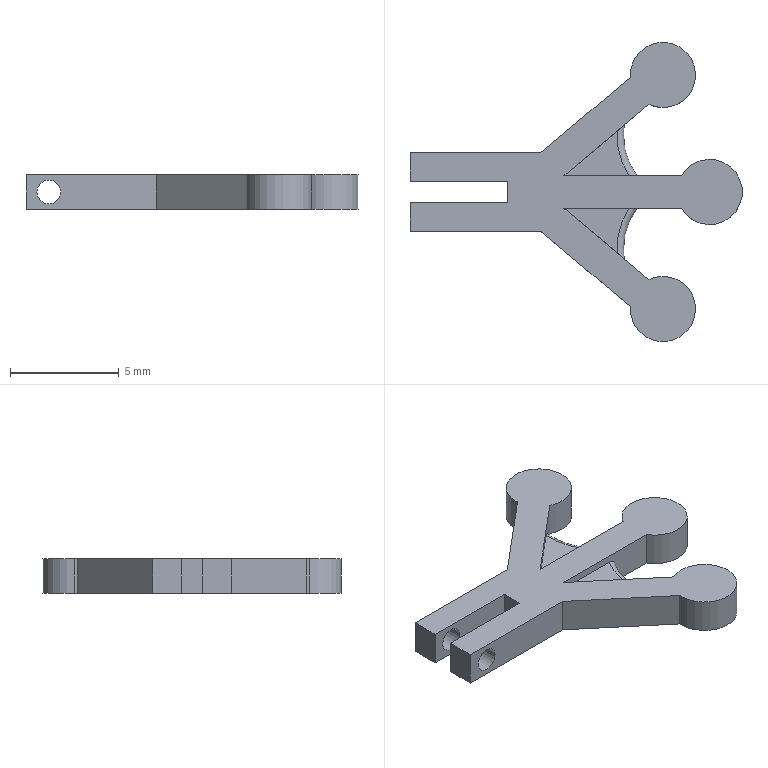Part | SolidWorks | features ICE 7, Extrusion 1, Fillet 1, Scale 1 | 1 solid | 38 faces | box 15.281 x 13.766 x 1.6 mm | volume 106.552 mm3 | plane 19 | cylinder 15 | torus 4 | commonest cylinder face diameters 3 x7 1.1 x4 6 x4
STEP:
#1=CARTESIAN_POINT('',(-0.2,-0.5,0.));
#2=VERTEX_POINT('',#1);
#3=CARTESIAN_POINT('',(-1.3,-0.5,0.));
#4=VERTEX_POINT('',#3);
#5=CARTESIAN_POINT('',(-0.75,-0.5,0.));
#6=DIRECTION('',(0.,1.,0.));
#7=DIRECTION('',(-1.,0.,0.));
#8=AXIS2_PLACEMENT_3D('',#5,#6,#7);
#9=CIRCLE('',#8,0.55);
#10=EDGE_CURVE('',#2,#4,#9,.T.);
#11=ORIENTED_EDGE('',*,*,#10,.T.);
#12=CARTESIAN_POINT('',(-1.3,-1.8,0.));
#13=VERTEX_POINT('',#12);
#14=CARTESIAN_POINT('',(-1.3,2.6,0.));
#15=DIRECTION('',(0.,-1.,0.));
#16=VECTOR('',#15,1000.);
#17=LINE('',#14,#16);
#18=EDGE_CURVE('',#4,#13,#17,.T.);
#19=ORIENTED_EDGE('',*,*,#18,.T.);
#20=CARTESIAN_POINT('',(-0.2,-1.8,0.));
#21=VERTEX_POINT('',#20);
#22=CARTESIAN_POINT('',(-0.75,-1.8,0.));
#23=DIRECTION('',(0.,-1.,0.));
#24=DIRECTION('',(1.,0.,0.));
#25=AXIS2_PLACEMENT_3D('',#22,#23,#24);
#26=CIRCLE('',#25,0.55);
#27=EDGE_CURVE('',#13,#21,#26,.T.);
#28=ORIENTED_EDGE('',*,*,#27,.T.);
#29=CARTESIAN_POINT('',(-0.2,2.6,0.));
#30=DIRECTION('',(0.,-1.,0.));
#31=VECTOR('',#30,1000.);
#32=LINE('',#29,#31);
#33=EDGE_CURVE('',#2,#21,#32,.T.);
#34=ORIENTED_EDGE('',*,*,#33,.F.);
#35=EDGE_LOOP('',(#11,#19,#28,#34));
#36=FACE_OUTER_BOUND('',#35,.T.);
#37=CARTESIAN_POINT('',(-0.75,2.6,0.));
#38=DIRECTION('',(0.,-1.,0.));
#39=DIRECTION('',(1.,0.,0.));
#40=AXIS2_PLACEMENT_3D('',#37,#38,#39);
#41=CYLINDRICAL_SURFACE('',#40,0.55);
#42=ADVANCED_FACE('',(#36),#41,.F.);
#43=CARTESIAN_POINT('',(-1.3,1.8,0.));
#44=VERTEX_POINT('',#43);
#45=CARTESIAN_POINT('',(-0.2,1.8,0.));
#46=VERTEX_POINT('',#45);
#47=CARTESIAN_POINT('',(-0.75,1.8,0.));
#48=DIRECTION('',(0.,-1.,0.));
#49=DIRECTION('',(1.,0.,0.));
#50=AXIS2_PLACEMENT_3D('',#47,#48,#49);
#51=CIRCLE('',#50,0.55);
#52=EDGE_CURVE('',#44,#46,#51,.T.);
#53=ORIENTED_EDGE('',*,*,#52,.F.);
#54=CARTESIAN_POINT('',(-1.3,0.5,0.));
#55=VERTEX_POINT('',#54);
#56=CARTESIAN_POINT('',(-1.3,2.6,0.));
#57=DIRECTION('',(0.,-1.,0.));
#58=VECTOR('',#57,1000.);
#59=LINE('',#56,#58);
#60=EDGE_CURVE('',#44,#55,#59,.T.);
#61=ORIENTED_EDGE('',*,*,#60,.T.);
#62=CARTESIAN_POINT('',(-0.2,0.5,0.));
#63=VERTEX_POINT('',#62);
#64=CARTESIAN_POINT('',(-0.75,0.5,0.));
#65=DIRECTION('',(0.,-1.,0.));
#66=DIRECTION('',(0.,0.,-1.));
#67=AXIS2_PLACEMENT_3D('',#64,#65,#66);
#68=CIRCLE('',#67,0.55);
#69=EDGE_CURVE('',#55,#63,#68,.T.);
#70=ORIENTED_EDGE('',*,*,#69,.T.);
#71=CARTESIAN_POINT('',(-0.2,2.6,0.));
#72=DIRECTION('',(0.,-1.,0.));
#73=VECTOR('',#72,1000.);
#74=LINE('',#71,#73);
#75=EDGE_CURVE('',#46,#63,#74,.T.);
#76=ORIENTED_EDGE('',*,*,#75,.F.);
#77=EDGE_LOOP('',(#53,#61,#70,#76));
#78=FACE_OUTER_BOUND('',#77,.T.);
#79=CARTESIAN_POINT('',(-0.75,2.6,0.));
#80=DIRECTION('',(0.,-1.,0.));
#81=DIRECTION('',(1.,0.,0.));
#82=AXIS2_PLACEMENT_3D('',#79,#80,#81);
#83=CYLINDRICAL_SURFACE('',#82,0.55);
#84=ADVANCED_FACE('',(#78),#83,.F.);
#85=CARTESIAN_POINT('',(8.644,-0.75,0.15));
#86=VERTEX_POINT('',#85);
#87=CARTESIAN_POINT('',(8.022,-2.578,0.15));
#88=VERTEX_POINT('',#87);
#89=CARTESIAN_POINT('',(11.022,-2.578,0.15));
#90=DIRECTION('',(0.,0.,1.));
#91=DIRECTION('',(1.,0.,0.));
#92=AXIS2_PLACEMENT_3D('',#89,#90,#91);
#93=CIRCLE('',#92,3.);
#94=EDGE_CURVE('',#86,#88,#93,.T.);
#95=ORIENTED_EDGE('',*,*,#94,.T.);
#96=CARTESIAN_POINT('',(8.022,-2.578,-0.15));
#97=VERTEX_POINT('',#96);
#98=CARTESIAN_POINT('',(8.022,-2.578,0.45));
#99=DIRECTION('',(0.,0.,-1.));
#100=VECTOR('',#99,1000.);
#101=LINE('',#98,#100);
#102=EDGE_CURVE('',#88,#97,#101,.T.);
#103=ORIENTED_EDGE('',*,*,#102,.T.);
#104=CARTESIAN_POINT('',(8.644,-0.75,-0.15));
#105=VERTEX_POINT('',#104);
#106=CARTESIAN_POINT('',(11.022,-2.578,-0.15));
#107=DIRECTION('',(0.,0.,-1.));
#108=DIRECTION('',(1.,0.,0.));
#109=AXIS2_PLACEMENT_3D('',#106,#107,#108);
#110=CIRCLE('',#109,3.);
#111=EDGE_CURVE('',#97,#105,#110,.T.);
#112=ORIENTED_EDGE('',*,*,#111,.T.);
#113=CARTESIAN_POINT('',(8.644,-0.75,0.45));
#114=DIRECTION('',(0.,0.,1.));
#115=VECTOR('',#114,1000.);
#116=LINE('',#113,#115);
#117=EDGE_CURVE('',#105,#86,#116,.T.);
#118=ORIENTED_EDGE('',*,*,#117,.T.);
#119=EDGE_LOOP('',(#95,#103,#112,#118));
#120=FACE_OUTER_BOUND('',#119,.T.);
#121=CARTESIAN_POINT('',(11.022,-2.578,0.45));
#122=DIRECTION('',(0.,0.,-1.));
#123=DIRECTION('',(-1.,0.,0.));
#124=AXIS2_PLACEMENT_3D('',#121,#122,#123);
#125=CYLINDRICAL_SURFACE('',#124,3.);
#126=ADVANCED_FACE('',(#120),#125,.F.);
#127=CARTESIAN_POINT('',(8.065,3.085,0.15));
#128=VERTEX_POINT('',#127);
#129=CARTESIAN_POINT('',(8.022,2.578,0.15));
#130=VERTEX_POINT('',#129);
#131=CARTESIAN_POINT('',(11.022,2.578,0.15));
#132=DIRECTION('',(0.,0.,1.));
#133=DIRECTION('',(1.,0.,0.));
#134=AXIS2_PLACEMENT_3D('',#131,#132,#133);
#135=CIRCLE('',#134,3.);
#136=EDGE_CURVE('',#128,#130,#135,.T.);
#137=ORIENTED_EDGE('',*,*,#136,.T.);
#138=CARTESIAN_POINT('',(8.022,2.578,-0.15));
#139=VERTEX_POINT('',#138);
#140=CARTESIAN_POINT('',(8.022,2.578,0.45));
#141=DIRECTION('',(0.,0.,-1.));
#142=VECTOR('',#141,1000.);
#143=LINE('',#140,#142);
#144=EDGE_CURVE('',#130,#139,#143,.T.);
#145=ORIENTED_EDGE('',*,*,#144,.T.);
#146=CARTESIAN_POINT('',(8.065,3.085,-0.15));
#147=VERTEX_POINT('',#146);
#148=CARTESIAN_POINT('',(11.022,2.578,-0.15));
#149=DIRECTION('',(0.,0.,-1.));
#150=DIRECTION('',(1.,0.,0.));
#151=AXIS2_PLACEMENT_3D('',#148,#149,#150);
#152=CIRCLE('',#151,3.);
#153=EDGE_CURVE('',#139,#147,#152,.T.);
#154=ORIENTED_EDGE('',*,*,#153,.T.);
#155=CARTESIAN_POINT('',(8.065,3.085,0.45));
#156=DIRECTION('',(0.,0.,-1.));
#157=VECTOR('',#156,1000.);
#158=LINE('',#155,#157);
#159=EDGE_CURVE('',#128,#147,#158,.T.);
#160=ORIENTED_EDGE('',*,*,#159,.F.);
#161=EDGE_LOOP('',(#137,#145,#154,#160));
#162=FACE_OUTER_BOUND('',#161,.T.);
#163=CARTESIAN_POINT('',(11.022,2.578,0.45));
#164=DIRECTION('',(0.,0.,-1.));
#165=DIRECTION('',(-1.,0.,0.));
#166=AXIS2_PLACEMENT_3D('',#163,#164,#165);
#167=CYLINDRICAL_SURFACE('',#166,3.);
#168=ADVANCED_FACE('',(#162),#167,.F.);
#169=CARTESIAN_POINT('',(11.332,5.383,0.8));
#170=VERTEX_POINT('',#169);
#171=CARTESIAN_POINT('',(8.332,5.383,0.8));
#172=VERTEX_POINT('',#171);
#173=CARTESIAN_POINT('',(9.832,5.383,0.8));
#174=DIRECTION('',(0.,0.,1.));
#175=DIRECTION('',(1.,0.,0.));
#176=AXIS2_PLACEMENT_3D('',#173,#174,#175);
#177=CIRCLE('',#176,1.5);
#178=EDGE_CURVE('',#170,#172,#177,.T.);
#179=ORIENTED_EDGE('',*,*,#178,.F.);
#180=CARTESIAN_POINT('',(11.332,5.383,-0.8));
#181=VERTEX_POINT('',#180);
#182=CARTESIAN_POINT('',(11.332,5.383,1.2));
#183=DIRECTION('',(0.,0.,-1.));
#184=VECTOR('',#183,1000.);
#185=LINE('',#182,#184);
#186=EDGE_CURVE('',#170,#181,#185,.T.);
#187=ORIENTED_EDGE('',*,*,#186,.T.);
#188=CARTESIAN_POINT('',(8.332,5.383,-0.8));
#189=VERTEX_POINT('',#188);
#190=CARTESIAN_POINT('',(9.832,5.383,-0.8));
#191=DIRECTION('',(0.,0.,-1.));
#192=DIRECTION('',(-1.,0.,0.));
#193=AXIS2_PLACEMENT_3D('',#190,#191,#192);
#194=CIRCLE('',#193,1.5);
#195=EDGE_CURVE('',#189,#181,#194,.T.);
#196=ORIENTED_EDGE('',*,*,#195,.F.);
#197=CARTESIAN_POINT('',(8.332,5.383,1.2));
#198=DIRECTION('',(0.,0.,-1.));
#199=VECTOR('',#198,1000.);
#200=LINE('',#197,#199);
#201=EDGE_CURVE('',#172,#189,#200,.T.);
#202=ORIENTED_EDGE('',*,*,#201,.F.);
#203=EDGE_LOOP('',(#179,#187,#196,#202));
#204=FACE_OUTER_BOUND('',#203,.T.);
#205=CARTESIAN_POINT('',(9.832,5.383,1.2));
#206=DIRECTION('',(0.,0.,-1.));
#207=DIRECTION('',(-1.,0.,0.));
#208=AXIS2_PLACEMENT_3D('',#205,#206,#207);
#209=CYLINDRICAL_SURFACE('',#208,1.5);
#210=ADVANCED_FACE('',(#204),#209,.T.);
#211=CARTESIAN_POINT('',(8.337,5.271,0.8));
#212=VERTEX_POINT('',#211);
#213=CARTESIAN_POINT('',(9.832,5.383,0.8));
#214=DIRECTION('',(0.,0.,1.));
#215=DIRECTION('',(1.,0.,0.));
#216=AXIS2_PLACEMENT_3D('',#213,#214,#215);
#217=CIRCLE('',#216,1.5);
#218=EDGE_CURVE('',#172,#212,#217,.T.);
#219=ORIENTED_EDGE('',*,*,#218,.F.);
#220=ORIENTED_EDGE('',*,*,#201,.T.);
#221=CARTESIAN_POINT('',(8.337,5.271,-0.8));
#222=VERTEX_POINT('',#221);
#223=CARTESIAN_POINT('',(9.832,5.383,-0.8));
#224=DIRECTION('',(0.,0.,-1.));
#225=DIRECTION('',(-1.,0.,0.));
#226=AXIS2_PLACEMENT_3D('',#223,#224,#225);
#227=CIRCLE('',#226,1.5);
#228=EDGE_CURVE('',#222,#189,#227,.T.);
#229=ORIENTED_EDGE('',*,*,#228,.F.);
#230=CARTESIAN_POINT('',(8.337,5.271,1.2));
#231=DIRECTION('',(0.,0.,-1.));
#232=VECTOR('',#231,1000.);
#233=LINE('',#230,#232);
#234=EDGE_CURVE('',#212,#222,#233,.T.);
#235=ORIENTED_EDGE('',*,*,#234,.F.);
#236=EDGE_LOOP('',(#219,#220,#229,#235));
#237=FACE_OUTER_BOUND('',#236,.T.);
#238=CARTESIAN_POINT('',(9.832,5.383,1.2));
#239=DIRECTION('',(0.,0.,-1.));
#240=DIRECTION('',(-1.,0.,0.));
#241=AXIS2_PLACEMENT_3D('',#238,#239,#240);
#242=CYLINDRICAL_SURFACE('',#241,1.5);
#243=ADVANCED_FACE('',(#237),#242,.T.);
#244=CARTESIAN_POINT('',(11.332,-5.383,0.8));
#245=VERTEX_POINT('',#244);
#246=CARTESIAN_POINT('',(9.189,-4.028,0.8));
#247=VERTEX_POINT('',#246);
#248=CARTESIAN_POINT('',(9.832,-5.383,0.8));
#249=DIRECTION('',(0.,0.,1.));
#250=DIRECTION('',(1.,0.,0.));
#251=AXIS2_PLACEMENT_3D('',#248,#249,#250);
#252=CIRCLE('',#251,1.5);
#253=EDGE_CURVE('',#245,#247,#252,.T.);
#254=ORIENTED_EDGE('',*,*,#253,.F.);
#255=CARTESIAN_POINT('',(11.332,-5.383,-0.8));
#256=VERTEX_POINT('',#255);
#257=CARTESIAN_POINT('',(11.332,-5.383,1.2));
#258=DIRECTION('',(0.,0.,-1.));
#259=VECTOR('',#258,1000.);
#260=LINE('',#257,#259);
#261=EDGE_CURVE('',#245,#256,#260,.T.);
#262=ORIENTED_EDGE('',*,*,#261,.T.);
#263=CARTESIAN_POINT('',(9.189,-4.028,-0.8));
#264=VERTEX_POINT('',#263);
#265=CARTESIAN_POINT('',(9.832,-5.383,-0.8));
#266=DIRECTION('',(0.,0.,-1.));
#267=DIRECTION('',(-1.,0.,0.));
#268=AXIS2_PLACEMENT_3D('',#265,#266,#267);
#269=CIRCLE('',#268,1.5);
#270=EDGE_CURVE('',#264,#256,#269,.T.);
#271=ORIENTED_EDGE('',*,*,#270,.F.);
#272=CARTESIAN_POINT('',(9.189,-4.028,1.2));
#273=DIRECTION('',(0.,0.,-1.));
#274=VECTOR('',#273,1000.);
#275=LINE('',#272,#274);
#276=EDGE_CURVE('',#247,#264,#275,.T.);
#277=ORIENTED_EDGE('',*,*,#276,.F.);
#278=EDGE_LOOP('',(#254,#262,#271,#277));
#279=FACE_OUTER_BOUND('',#278,.T.);
#280=CARTESIAN_POINT('',(9.832,-5.383,1.2));
#281=DIRECTION('',(0.,0.,-1.));
#282=DIRECTION('',(-1.,0.,0.));
#283=AXIS2_PLACEMENT_3D('',#280,#281,#282);
#284=CYLINDRICAL_SURFACE('',#283,1.5);
#285=ADVANCED_FACE('',(#279),#284,.T.);
#286=ORIENTED_EDGE('',*,*,#261,.F.);
#287=CARTESIAN_POINT('',(8.332,-5.383,0.8));
#288=VERTEX_POINT('',#287);
#289=CARTESIAN_POINT('',(9.832,-5.383,0.8));
#290=DIRECTION('',(0.,0.,1.));
#291=DIRECTION('',(1.,0.,0.));
#292=AXIS2_PLACEMENT_3D('',#289,#290,#291);
#293=CIRCLE('',#292,1.5);
#294=EDGE_CURVE('',#288,#245,#293,.T.);
#295=ORIENTED_EDGE('',*,*,#294,.F.);
#296=CARTESIAN_POINT('',(8.332,-5.383,-0.8));
#297=VERTEX_POINT('',#296);
#298=CARTESIAN_POINT('',(8.332,-5.383,1.2));
#299=DIRECTION('',(0.,0.,-1.));
#300=VECTOR('',#299,1000.);
#301=LINE('',#298,#300);
#302=EDGE_CURVE('',#288,#297,#301,.T.);
#303=ORIENTED_EDGE('',*,*,#302,.T.);
#304=CARTESIAN_POINT('',(9.832,-5.383,-0.8));
#305=DIRECTION('',(0.,0.,-1.));
#306=DIRECTION('',(-1.,0.,0.));
#307=AXIS2_PLACEMENT_3D('',#304,#305,#306);
#308=CIRCLE('',#307,1.5);
#309=EDGE_CURVE('',#256,#297,#308,.T.);
#310=ORIENTED_EDGE('',*,*,#309,.F.);
#311=EDGE_LOOP('',(#286,#295,#303,#310));
#312=FACE_OUTER_BOUND('',#311,.T.);
#313=CARTESIAN_POINT('',(9.832,-5.383,1.2));
#314=DIRECTION('',(0.,0.,-1.));
#315=DIRECTION('',(-1.,0.,0.));
#316=AXIS2_PLACEMENT_3D('',#313,#314,#315);
#317=CYLINDRICAL_SURFACE('',#316,1.5);
#318=ADVANCED_FACE('',(#312),#317,.T.);
#319=CARTESIAN_POINT('',(-1.8,0.5,-0.8));
#320=VERTEX_POINT('',#319);
#321=CARTESIAN_POINT('',(-1.8,1.8,-0.8));
#322=VERTEX_POINT('',#321);
#323=CARTESIAN_POINT('',(-1.8,0.,-0.8));
#324=DIRECTION('',(0.,1.,0.));
#325=VECTOR('',#324,1000.);
#326=LINE('',#323,#325);
#327=EDGE_CURVE('',#320,#322,#326,.T.);
#328=ORIENTED_EDGE('',*,*,#327,.F.);
#329=CARTESIAN_POINT('',(-1.8,0.5,0.8));
#330=VERTEX_POINT('',#329);
#331=CARTESIAN_POINT('',(-1.8,0.5,-5.301));
#332=DIRECTION('',(0.,0.,1.));
#333=VECTOR('',#332,1000.);
#334=LINE('',#331,#333);
#335=EDGE_CURVE('',#320,#330,#334,.T.);
#336=ORIENTED_EDGE('',*,*,#335,.T.);
#337=CARTESIAN_POINT('',(-1.8,1.8,0.8));
#338=VERTEX_POINT('',#337);
#339=CARTESIAN_POINT('',(-1.8,0.,0.8));
#340=DIRECTION('',(0.,-1.,0.));
#341=VECTOR('',#340,1000.);
#342=LINE('',#339,#341);
#343=EDGE_CURVE('',#338,#330,#342,.T.);
#344=ORIENTED_EDGE('',*,*,#343,.F.);
#345=CARTESIAN_POINT('',(-1.8,1.8,1.2));
#346=DIRECTION('',(0.,0.,-1.));
#347=VECTOR('',#346,1000.);
#348=LINE('',#345,#347);
#349=EDGE_CURVE('',#338,#322,#348,.T.);
#350=ORIENTED_EDGE('',*,*,#349,.T.);
#351=EDGE_LOOP('',(#328,#336,#344,#350));
#352=FACE_OUTER_BOUND('',#351,.T.);
#353=CARTESIAN_POINT('',(-1.8,0.,1.2));
#354=DIRECTION('',(1.,0.,0.));
#355=DIRECTION('',(0.,0.,-1.));
#356=AXIS2_PLACEMENT_3D('',#353,#354,#355);
#357=PLANE('',#356);
#358=ADVANCED_FACE('',(#352),#357,.F.);
#359=CARTESIAN_POINT('',(-0.75,-1.8,0.));
#360=DIRECTION('',(0.,-1.,0.));
#361=DIRECTION('',(1.,0.,0.));
#362=AXIS2_PLACEMENT_3D('',#359,#360,#361);
#363=CIRCLE('',#362,0.55);
#364=EDGE_CURVE('',#21,#13,#363,.T.);
#365=ORIENTED_EDGE('',*,*,#364,.F.);
#366=ORIENTED_EDGE('',*,*,#27,.F.);
#367=EDGE_LOOP('',(#365,#366));
#368=FACE_BOUND('',#367,.T.);
#369=CARTESIAN_POINT('',(4.2,-1.8,-0.8));
#370=VERTEX_POINT('',#369);
#371=CARTESIAN_POINT('',(-1.8,-1.8,-0.8));
#372=VERTEX_POINT('',#371);
#373=CARTESIAN_POINT('',(-1.8,-1.8,-0.8));
#374=DIRECTION('',(-1.,0.,0.));
#375=VECTOR('',#374,1000.);
#376=LINE('',#373,#375);
#377=EDGE_CURVE('',#370,#372,#376,.T.);
#378=ORIENTED_EDGE('',*,*,#377,.F.);
#379=CARTESIAN_POINT('',(4.2,-1.8,0.8));
#380=VERTEX_POINT('',#379);
#381=CARTESIAN_POINT('',(4.2,-1.8,1.2));
#382=DIRECTION('',(0.,0.,-1.));
#383=VECTOR('',#382,1000.);
#384=LINE('',#381,#383);
#385=EDGE_CURVE('',#380,#370,#384,.T.);
#386=ORIENTED_EDGE('',*,*,#385,.F.);
#387=CARTESIAN_POINT('',(-1.8,-1.8,0.8));
#388=VERTEX_POINT('',#387);
#389=CARTESIAN_POINT('',(-1.8,-1.8,0.8));
#390=DIRECTION('',(1.,0.,0.));
#391=VECTOR('',#390,1000.);
#392=LINE('',#389,#391);
#393=EDGE_CURVE('',#388,#380,#392,.T.);
#394=ORIENTED_EDGE('',*,*,#393,.F.);
#395=CARTESIAN_POINT('',(-1.8,-1.8,1.2));
#396=DIRECTION('',(0.,0.,-1.));
#397=VECTOR('',#396,1000.);
#398=LINE('',#395,#397);
#399=EDGE_CURVE('',#388,#372,#398,.T.);
#400=ORIENTED_EDGE('',*,*,#399,.T.);
#401=EDGE_LOOP('',(#378,#386,#394,#400));
#402=FACE_OUTER_BOUND('',#401,.T.);
#403=CARTESIAN_POINT('',(-1.8,-1.8,1.2));
#404=DIRECTION('',(0.,1.,0.));
#405=DIRECTION('',(-1.,0.,0.));
#406=AXIS2_PLACEMENT_3D('',#403,#404,#405);
#407=PLANE('',#406);
#408=ADVANCED_FACE('',(#368,#402),#407,.F.);
#409=CARTESIAN_POINT('',(8.337,-5.271,-0.8));
#410=VERTEX_POINT('',#409);
#411=CARTESIAN_POINT('',(4.2,-1.8,-0.8));
#412=DIRECTION('',(-0.766,0.6428,0.));
#413=VECTOR('',#412,1000.);
#414=LINE('',#411,#413);
#415=EDGE_CURVE('',#410,#370,#414,.T.);
#416=ORIENTED_EDGE('',*,*,#415,.F.);
#417=CARTESIAN_POINT('',(8.337,-5.271,0.8));
#418=VERTEX_POINT('',#417);
#419=CARTESIAN_POINT('',(8.337,-5.271,1.2));
#420=DIRECTION('',(0.,0.,-1.));
#421=VECTOR('',#420,1000.);
#422=LINE('',#419,#421);
#423=EDGE_CURVE('',#418,#410,#422,.T.);
#424=ORIENTED_EDGE('',*,*,#423,.F.);
#425=CARTESIAN_POINT('',(4.2,-1.8,0.8));
#426=DIRECTION('',(0.766,-0.6428,0.));
#427=VECTOR('',#426,1000.);
#428=LINE('',#425,#427);
#429=EDGE_CURVE('',#380,#418,#428,.T.);
#430=ORIENTED_EDGE('',*,*,#429,.F.);
#431=ORIENTED_EDGE('',*,*,#385,.T.);
#432=EDGE_LOOP('',(#416,#424,#430,#431));
#433=FACE_OUTER_BOUND('',#432,.T.);
#434=CARTESIAN_POINT('',(4.2,-1.8,1.2));
#435=DIRECTION('',(0.6428,0.766,0.));
#436=DIRECTION('',(-0.766,0.6428,0.));
#437=AXIS2_PLACEMENT_3D('',#434,#435,#436);
#438=PLANE('',#437);
#439=ADVANCED_FACE('',(#433),#438,.F.);
#440=ORIENTED_EDGE('',*,*,#302,.F.);
#441=CARTESIAN_POINT('',(9.832,-5.383,0.8));
#442=DIRECTION('',(0.,0.,1.));
#443=DIRECTION('',(1.,0.,0.));
#444=AXIS2_PLACEMENT_3D('',#441,#442,#443);
#445=CIRCLE('',#444,1.5);
#446=EDGE_CURVE('',#418,#288,#445,.T.);
#447=ORIENTED_EDGE('',*,*,#446,.F.);
#448=ORIENTED_EDGE('',*,*,#423,.T.);
#449=CARTESIAN_POINT('',(9.832,-5.383,-0.8));
#450=DIRECTION('',(0.,0.,-1.));
#451=DIRECTION('',(-1.,0.,0.));
#452=AXIS2_PLACEMENT_3D('',#449,#450,#451);
#453=CIRCLE('',#452,1.5);
#454=EDGE_CURVE('',#297,#410,#453,.T.);
#455=ORIENTED_EDGE('',*,*,#454,.F.);
#456=EDGE_LOOP('',(#440,#447,#448,#455));
#457=FACE_OUTER_BOUND('',#456,.T.);
#458=CARTESIAN_POINT('',(9.832,-5.383,1.2));
#459=DIRECTION('',(0.,0.,-1.));
#460=DIRECTION('',(-1.,0.,0.));
#461=AXIS2_PLACEMENT_3D('',#458,#459,#460);
#462=CYLINDRICAL_SURFACE('',#461,1.5);
#463=ADVANCED_FACE('',(#457),#462,.T.);
#464=CARTESIAN_POINT('',(5.282,-0.75,-0.8));
#465=VERTEX_POINT('',#464);
#466=CARTESIAN_POINT('',(9.189,-4.028,-0.8));
#467=DIRECTION('',(0.766,-0.6428,0.));
#468=VECTOR('',#467,1000.);
#469=LINE('',#466,#468);
#470=EDGE_CURVE('',#465,#264,#469,.T.);
#471=ORIENTED_EDGE('',*,*,#470,.F.);
#472=CARTESIAN_POINT('',(5.282,-0.75,-0.45));
#473=VERTEX_POINT('',#472);
#474=CARTESIAN_POINT('',(5.282,-0.75,1.2));
#475=DIRECTION('',(0.,0.,-1.));
#476=VECTOR('',#475,1000.);
#477=LINE('',#474,#476);
#478=EDGE_CURVE('',#473,#465,#477,.T.);
#479=ORIENTED_EDGE('',*,*,#478,.F.);
#480=CARTESIAN_POINT('',(7.73,-2.804,-0.45));
#481=VERTEX_POINT('',#480);
#482=CARTESIAN_POINT('',(4.388,0.,-0.45));
#483=DIRECTION('',(0.766,-0.6428,0.));
#484=VECTOR('',#483,1000.);
#485=LINE('',#482,#484);
#486=EDGE_CURVE('',#473,#481,#485,.T.);
#487=ORIENTED_EDGE('',*,*,#486,.T.);
#488=CARTESIAN_POINT('',(8.065,-3.085,-0.15));
#489=VERTEX_POINT('',#488);
#490=CARTESIAN_POINT('',(7.73,-2.804,-0.45));
#491=CARTESIAN_POINT('',(7.805,-2.867,-0.45));
#492=CARTESIAN_POINT('',(7.879,-2.929,-0.4267));
#493=CARTESIAN_POINT('',(7.975,-3.01,-0.3545));
#494=CARTESIAN_POINT('',(8.005,-3.035,-0.3237));
#495=CARTESIAN_POINT('',(8.05,-3.073,-0.2463));
#496=CARTESIAN_POINT('',(8.065,-3.085,-0.1992));
#497=CARTESIAN_POINT('',(8.065,-3.085,-0.15));
#498=B_SPLINE_CURVE_WITH_KNOTS('',3,(#490,#491,#492,#493,#494,#495,#496,#497),.UNSPECIFIED.,.F.,.F.,(4,2,2,4),(0.,0.0002886,0.000433,0.0005773),.UNSPECIFIED.);
#499=EDGE_CURVE('',#481,#489,#498,.T.);
#500=ORIENTED_EDGE('',*,*,#499,.T.);
#501=CARTESIAN_POINT('',(8.065,-3.085,0.15));
#502=VERTEX_POINT('',#501);
#503=CARTESIAN_POINT('',(8.065,-3.085,0.45));
#504=DIRECTION('',(0.,0.,-1.));
#505=VECTOR('',#504,1000.);
#506=LINE('',#503,#505);
#507=EDGE_CURVE('',#502,#489,#506,.T.);
#508=ORIENTED_EDGE('',*,*,#507,.F.);
#509=CARTESIAN_POINT('',(7.73,-2.804,0.45));
#510=VERTEX_POINT('',#509);
#511=CARTESIAN_POINT('',(8.065,-3.085,0.15));
#512=CARTESIAN_POINT('',(8.065,-3.085,0.1993));
#513=CARTESIAN_POINT('',(8.051,-3.073,0.2459));
#514=CARTESIAN_POINT('',(8.005,-3.035,0.3235));
#515=CARTESIAN_POINT('',(7.975,-3.01,0.3542));
#516=CARTESIAN_POINT('',(7.879,-2.929,0.4268));
#517=CARTESIAN_POINT('',(7.805,-2.867,0.45));
#518=CARTESIAN_POINT('',(7.73,-2.804,0.45));
#519=B_SPLINE_CURVE_WITH_KNOTS('',3,(#511,#512,#513,#514,#515,#516,#517,#518),.UNSPECIFIED.,.F.,.F.,(4,2,2,4),(0.,0.000145,0.0002899,0.0005799),.UNSPECIFIED.);
#520=EDGE_CURVE('',#502,#510,#519,.T.);
#521=ORIENTED_EDGE('',*,*,#520,.T.);
#522=CARTESIAN_POINT('',(5.282,-0.75,0.45));
#523=VERTEX_POINT('',#522);
#524=CARTESIAN_POINT('',(4.388,0.,0.45));
#525=DIRECTION('',(0.766,-0.6428,0.));
#526=VECTOR('',#525,1000.);
#527=LINE('',#524,#526);
#528=EDGE_CURVE('',#523,#510,#527,.T.);
#529=ORIENTED_EDGE('',*,*,#528,.F.);
#530=CARTESIAN_POINT('',(5.282,-0.75,0.8));
#531=VERTEX_POINT('',#530);
#532=CARTESIAN_POINT('',(5.282,-0.75,1.2));
#533=DIRECTION('',(0.,0.,-1.));
#534=VECTOR('',#533,1000.);
#535=LINE('',#532,#534);
#536=EDGE_CURVE('',#531,#523,#535,.T.);
#537=ORIENTED_EDGE('',*,*,#536,.F.);
#538=CARTESIAN_POINT('',(9.189,-4.028,0.8));
#539=DIRECTION('',(-0.766,0.6428,0.));
#540=VECTOR('',#539,1000.);
#541=LINE('',#538,#540);
#542=EDGE_CURVE('',#247,#531,#541,.T.);
#543=ORIENTED_EDGE('',*,*,#542,.F.);
#544=ORIENTED_EDGE('',*,*,#276,.T.);
#545=EDGE_LOOP('',(#471,#479,#487,#500,#508,#521,#529,#537,#543,#544));
#546=FACE_OUTER_BOUND('',#545,.T.);
#547=CARTESIAN_POINT('',(9.189,-4.028,1.2));
#548=DIRECTION('',(-0.6428,-0.766,0.));
#549=DIRECTION('',(0.766,-0.6428,0.));
#550=AXIS2_PLACEMENT_3D('',#547,#548,#549);
#551=PLANE('',#550);
#552=ADVANCED_FACE('',(#546),#551,.F.);
#553=CARTESIAN_POINT('',(10.682,-0.75,-0.8));
#554=VERTEX_POINT('',#553);
#555=CARTESIAN_POINT('',(5.282,-0.75,-0.8));
#556=DIRECTION('',(-1.,0.,0.));
#557=VECTOR('',#556,1000.);
#558=LINE('',#555,#557);
#559=EDGE_CURVE('',#554,#465,#558,.T.);
#560=ORIENTED_EDGE('',*,*,#559,.F.);
#561=CARTESIAN_POINT('',(10.682,-0.75,0.8));
#562=VERTEX_POINT('',#561);
#563=CARTESIAN_POINT('',(10.682,-0.75,1.2));
#564=DIRECTION('',(0.,0.,-1.));
#565=VECTOR('',#564,1000.);
#566=LINE('',#563,#565);
#567=EDGE_CURVE('',#562,#554,#566,.T.);
#568=ORIENTED_EDGE('',*,*,#567,.F.);
#569=CARTESIAN_POINT('',(5.282,-0.75,0.8));
#570=DIRECTION('',(1.,0.,0.));
#571=VECTOR('',#570,1000.);
#572=LINE('',#569,#571);
#573=EDGE_CURVE('',#531,#562,#572,.T.);
#574=ORIENTED_EDGE('',*,*,#573,.F.);
#575=ORIENTED_EDGE('',*,*,#536,.T.);
#576=CARTESIAN_POINT('',(8.275,-0.75,0.45));
#577=VERTEX_POINT('',#576);
#578=CARTESIAN_POINT('',(5.282,-0.75,0.45));
#579=DIRECTION('',(1.,0.,0.));
#580=VECTOR('',#579,1000.);
#581=LINE('',#578,#580);
#582=EDGE_CURVE('',#523,#577,#581,.T.);
#583=ORIENTED_EDGE('',*,*,#582,.T.);
#584=CARTESIAN_POINT('',(8.275,-0.75,0.45));
#585=CARTESIAN_POINT('',(8.363,-0.75,0.45));
#586=CARTESIAN_POINT('',(8.45,-0.75,0.4237));
#587=CARTESIAN_POINT('',(8.591,-0.75,0.3207));
#588=CARTESIAN_POINT('',(8.644,-0.75,0.2389));
#589=CARTESIAN_POINT('',(8.644,-0.75,0.15));
#590=B_SPLINE_CURVE_WITH_KNOTS('',3,(#584,#585,#586,#587,#588,#589),.UNSPECIFIED.,.F.,.F.,(4,2,4),(0.,0.0002609,0.0005217),.UNSPECIFIED.);
#591=EDGE_CURVE('',#577,#86,#590,.T.);
#592=ORIENTED_EDGE('',*,*,#591,.T.);
#593=ORIENTED_EDGE('',*,*,#117,.F.);
#594=CARTESIAN_POINT('',(8.275,-0.75,-0.45));
#595=VERTEX_POINT('',#594);
#596=CARTESIAN_POINT('',(8.644,-0.75,-0.15));
#597=CARTESIAN_POINT('',(8.644,-0.75,-0.2385));
#598=CARTESIAN_POINT('',(8.592,-0.75,-0.3196));
#599=CARTESIAN_POINT('',(8.45,-0.75,-0.424));
#600=CARTESIAN_POINT('',(8.363,-0.75,-0.45));
#601=CARTESIAN_POINT('',(8.275,-0.75,-0.45));
#602=B_SPLINE_CURVE_WITH_KNOTS('',3,(#596,#597,#598,#599,#600,#601),.UNSPECIFIED.,.F.,.F.,(4,2,4),(0.,0.0002613,0.0005227),.UNSPECIFIED.);
#603=EDGE_CURVE('',#105,#595,#602,.T.);
#604=ORIENTED_EDGE('',*,*,#603,.T.);
#605=CARTESIAN_POINT('',(5.282,-0.75,-0.45));
#606=DIRECTION('',(1.,0.,0.));
#607=VECTOR('',#606,1000.);
#608=LINE('',#605,#607);
#609=EDGE_CURVE('',#473,#595,#608,.T.);
#610=ORIENTED_EDGE('',*,*,#609,.F.);
#611=ORIENTED_EDGE('',*,*,#478,.T.);
#612=EDGE_LOOP('',(#560,#568,#574,#575,#583,#592,#593,#604,#610,#611));
#613=FACE_OUTER_BOUND('',#612,.T.);
#614=CARTESIAN_POINT('',(5.282,-0.75,1.2));
#615=DIRECTION('',(0.,1.,0.));
#616=DIRECTION('',(0.,0.,1.));
#617=AXIS2_PLACEMENT_3D('',#614,#615,#616);
#618=PLANE('',#617);
#619=ADVANCED_FACE('',(#613),#618,.F.);
#620=CARTESIAN_POINT('',(10.682,0.75,-0.8));
#621=VERTEX_POINT('',#620);
#622=CARTESIAN_POINT('',(11.981,0.,-0.8));
#623=DIRECTION('',(0.,0.,-1.));
#624=DIRECTION('',(-1.,0.,0.));
#625=AXIS2_PLACEMENT_3D('',#622,#623,#624);
#626=CIRCLE('',#625,1.5);
#627=EDGE_CURVE('',#621,#554,#626,.T.);
#628=ORIENTED_EDGE('',*,*,#627,.F.);
#629=CARTESIAN_POINT('',(10.682,0.75,0.8));
#630=VERTEX_POINT('',#629);
#631=CARTESIAN_POINT('',(10.682,0.75,1.2));
#632=DIRECTION('',(0.,0.,-1.));
#633=VECTOR('',#632,1000.);
#634=LINE('',#631,#633);
#635=EDGE_CURVE('',#630,#621,#634,.T.);
#636=ORIENTED_EDGE('',*,*,#635,.F.);
#637=CARTESIAN_POINT('',(11.981,0.,0.8));
#638=DIRECTION('',(0.,0.,1.));
#639=DIRECTION('',(1.,0.,0.));
#640=AXIS2_PLACEMENT_3D('',#637,#638,#639);
#641=CIRCLE('',#640,1.5);
#642=EDGE_CURVE('',#562,#630,#641,.T.);
#643=ORIENTED_EDGE('',*,*,#642,.F.);
#644=ORIENTED_EDGE('',*,*,#567,.T.);
#645=EDGE_LOOP('',(#628,#636,#643,#644));
#646=FACE_OUTER_BOUND('',#645,.T.);
#647=CARTESIAN_POINT('',(11.981,0.,1.2));
#648=DIRECTION('',(0.,0.,-1.));
#649=DIRECTION('',(-1.,0.,0.));
#650=AXIS2_PLACEMENT_3D('',#647,#648,#649);
#651=CYLINDRICAL_SURFACE('',#650,1.5);
#652=ADVANCED_FACE('',(#646),#651,.T.);
#653=CARTESIAN_POINT('',(5.282,0.75,-0.8));
#654=VERTEX_POINT('',#653);
#655=CARTESIAN_POINT('',(5.282,0.75,-0.8));
#656=DIRECTION('',(1.,0.,0.));
#657=VECTOR('',#656,1000.);
#658=LINE('',#655,#657);
#659=EDGE_CURVE('',#654,#621,#658,.T.);
#660=ORIENTED_EDGE('',*,*,#659,.F.);
#661=CARTESIAN_POINT('',(5.282,0.75,-0.45));
#662=VERTEX_POINT('',#661);
#663=CARTESIAN_POINT('',(5.282,0.75,1.2));
#664=DIRECTION('',(0.,0.,-1.));
#665=VECTOR('',#664,1000.);
#666=LINE('',#663,#665);
#667=EDGE_CURVE('',#662,#654,#666,.T.);
#668=ORIENTED_EDGE('',*,*,#667,.F.);
#669=CARTESIAN_POINT('',(8.275,0.75,-0.45));
#670=VERTEX_POINT('',#669);
#671=CARTESIAN_POINT('',(5.282,0.75,-0.45));
#672=DIRECTION('',(-1.,0.,0.));
#673=VECTOR('',#672,1000.);
#674=LINE('',#671,#673);
#675=EDGE_CURVE('',#670,#662,#674,.T.);
#676=ORIENTED_EDGE('',*,*,#675,.F.);
#677=CARTESIAN_POINT('',(8.644,0.75,-0.15));
#678=VERTEX_POINT('',#677);
#679=CARTESIAN_POINT('',(8.275,0.75,-0.45));
#680=CARTESIAN_POINT('',(8.363,0.75,-0.45));
#681=CARTESIAN_POINT('',(8.45,0.75,-0.4237));
#682=CARTESIAN_POINT('',(8.591,0.75,-0.3207));
#683=CARTESIAN_POINT('',(8.644,0.75,-0.2389));
#684=CARTESIAN_POINT('',(8.644,0.75,-0.15));
#685=B_SPLINE_CURVE_WITH_KNOTS('',3,(#679,#680,#681,#682,#683,#684),.UNSPECIFIED.,.F.,.F.,(4,2,4),(0.,0.0002609,0.0005217),.UNSPECIFIED.);
#686=EDGE_CURVE('',#670,#678,#685,.T.);
#687=ORIENTED_EDGE('',*,*,#686,.T.);
#688=CARTESIAN_POINT('',(8.644,0.75,0.15));
#689=VERTEX_POINT('',#688);
#690=CARTESIAN_POINT('',(8.644,0.75,0.45));
#691=DIRECTION('',(0.,0.,-1.));
#692=VECTOR('',#691,1000.);
#693=LINE('',#690,#692);
#694=EDGE_CURVE('',#689,#678,#693,.T.);
#695=ORIENTED_EDGE('',*,*,#694,.F.);
#696=CARTESIAN_POINT('',(8.275,0.75,0.45));
#697=VERTEX_POINT('',#696);
#698=CARTESIAN_POINT('',(8.644,0.75,0.15));
#699=CARTESIAN_POINT('',(8.644,0.75,0.2385));
#700=CARTESIAN_POINT('',(8.592,0.75,0.3196));
#701=CARTESIAN_POINT('',(8.45,0.75,0.424));
#702=CARTESIAN_POINT('',(8.363,0.75,0.45));
#703=CARTESIAN_POINT('',(8.275,0.75,0.45));
#704=B_SPLINE_CURVE_WITH_KNOTS('',3,(#698,#699,#700,#701,#702,#703),.UNSPECIFIED.,.F.,.F.,(4,2,4),(0.,0.0002613,0.0005227),.UNSPECIFIED.);
#705=EDGE_CURVE('',#689,#697,#704,.T.);
#706=ORIENTED_EDGE('',*,*,#705,.T.);
#707=CARTESIAN_POINT('',(5.282,0.75,0.45));
#708=VERTEX_POINT('',#707);
#709=CARTESIAN_POINT('',(5.282,0.75,0.45));
#710=DIRECTION('',(-1.,0.,0.));
#711=VECTOR('',#710,1000.);
#712=LINE('',#709,#711);
#713=EDGE_CURVE('',#697,#708,#712,.T.);
#714=ORIENTED_EDGE('',*,*,#713,.T.);
#715=CARTESIAN_POINT('',(5.282,0.75,0.8));
#716=VERTEX_POINT('',#715);
#717=CARTESIAN_POINT('',(5.282,0.75,1.2));
#718=DIRECTION('',(0.,0.,-1.));
#719=VECTOR('',#718,1000.);
#720=LINE('',#717,#719);
#721=EDGE_CURVE('',#716,#708,#720,.T.);
#722=ORIENTED_EDGE('',*,*,#721,.F.);
#723=CARTESIAN_POINT('',(5.282,0.75,0.8));
#724=DIRECTION('',(-1.,0.,0.));
#725=VECTOR('',#724,1000.);
#726=LINE('',#723,#725);
#727=EDGE_CURVE('',#630,#716,#726,.T.);
#728=ORIENTED_EDGE('',*,*,#727,.F.);
#729=ORIENTED_EDGE('',*,*,#635,.T.);
#730=EDGE_LOOP('',(#660,#668,#676,#687,#695,#706,#714,#722,#728,#729));
#731=FACE_OUTER_BOUND('',#730,.T.);
#732=CARTESIAN_POINT('',(5.282,0.75,1.2));
#733=DIRECTION('',(0.,-1.,0.));
#734=DIRECTION('',(0.,0.,-1.));
#735=AXIS2_PLACEMENT_3D('',#732,#733,#734);
#736=PLANE('',#735);
#737=ADVANCED_FACE('',(#731),#736,.F.);
#738=CARTESIAN_POINT('',(9.189,4.028,-0.8));
#739=VERTEX_POINT('',#738);
#740=CARTESIAN_POINT('',(9.189,4.028,-0.8));
#741=DIRECTION('',(-0.766,-0.6428,0.));
#742=VECTOR('',#741,1000.);
#743=LINE('',#740,#742);
#744=EDGE_CURVE('',#739,#654,#743,.T.);
#745=ORIENTED_EDGE('',*,*,#744,.F.);
#746=CARTESIAN_POINT('',(9.189,4.028,0.8));
#747=VERTEX_POINT('',#746);
#748=CARTESIAN_POINT('',(9.189,4.028,1.2));
#749=DIRECTION('',(0.,0.,-1.));
#750=VECTOR('',#749,1000.);
#751=LINE('',#748,#750);
#752=EDGE_CURVE('',#747,#739,#751,.T.);
#753=ORIENTED_EDGE('',*,*,#752,.F.);
#754=CARTESIAN_POINT('',(9.189,4.028,0.8));
#755=DIRECTION('',(0.766,0.6428,0.));
#756=VECTOR('',#755,1000.);
#757=LINE('',#754,#756);
#758=EDGE_CURVE('',#716,#747,#757,.T.);
#759=ORIENTED_EDGE('',*,*,#758,.F.);
#760=ORIENTED_EDGE('',*,*,#721,.T.);
#761=CARTESIAN_POINT('',(7.73,2.804,0.45));
#762=VERTEX_POINT('',#761);
#763=CARTESIAN_POINT('',(8.065,3.085,0.45));
#764=DIRECTION('',(-0.766,-0.6428,0.));
#765=VECTOR('',#764,1000.);
#766=LINE('',#763,#765);
#767=EDGE_CURVE('',#762,#708,#766,.T.);
#768=ORIENTED_EDGE('',*,*,#767,.F.);
#769=CARTESIAN_POINT('',(7.73,2.804,0.45));
#770=CARTESIAN_POINT('',(7.805,2.867,0.45));
#771=CARTESIAN_POINT('',(7.879,2.929,0.4267));
#772=CARTESIAN_POINT('',(7.975,3.01,0.3545));
#773=CARTESIAN_POINT('',(8.005,3.035,0.3237));
#774=CARTESIAN_POINT('',(8.05,3.073,0.2463));
#775=CARTESIAN_POINT('',(8.065,3.085,0.1992));
#776=CARTESIAN_POINT('',(8.065,3.085,0.15));
#777=B_SPLINE_CURVE_WITH_KNOTS('',3,(#769,#770,#771,#772,#773,#774,#775,#776),.UNSPECIFIED.,.F.,.F.,(4,2,2,4),(0.,0.0002886,0.000433,0.0005773),.UNSPECIFIED.);
#778=EDGE_CURVE('',#762,#128,#777,.T.);
#779=ORIENTED_EDGE('',*,*,#778,.T.);
#780=ORIENTED_EDGE('',*,*,#159,.T.);
#781=CARTESIAN_POINT('',(7.73,2.804,-0.45));
#782=VERTEX_POINT('',#781);
#783=CARTESIAN_POINT('',(8.065,3.085,-0.15));
#784=CARTESIAN_POINT('',(8.065,3.085,-0.1993));
#785=CARTESIAN_POINT('',(8.051,3.073,-0.2459));
#786=CARTESIAN_POINT('',(8.005,3.035,-0.3235));
#787=CARTESIAN_POINT('',(7.975,3.01,-0.3542));
#788=CARTESIAN_POINT('',(7.879,2.929,-0.4268));
#789=CARTESIAN_POINT('',(7.805,2.867,-0.45));
#790=CARTESIAN_POINT('',(7.73,2.804,-0.45));
#791=B_SPLINE_CURVE_WITH_KNOTS('',3,(#783,#784,#785,#786,#787,#788,#789,#790),.UNSPECIFIED.,.F.,.F.,(4,2,2,4),(0.,0.000145,0.0002899,0.0005799),.UNSPECIFIED.);
#792=EDGE_CURVE('',#147,#782,#791,.T.);
#793=ORIENTED_EDGE('',*,*,#792,.T.);
#794=CARTESIAN_POINT('',(8.065,3.085,-0.45));
#795=DIRECTION('',(-0.766,-0.6428,0.));
#796=VECTOR('',#795,1000.);
#797=LINE('',#794,#796);
#798=EDGE_CURVE('',#782,#662,#797,.T.);
#799=ORIENTED_EDGE('',*,*,#798,.T.);
#800=ORIENTED_EDGE('',*,*,#667,.T.);
#801=EDGE_LOOP('',(#745,#753,#759,#760,#768,#779,#780,#793,#799,#800));
#802=FACE_OUTER_BOUND('',#801,.T.);
#803=CARTESIAN_POINT('',(9.189,4.028,1.2));
#804=DIRECTION('',(-0.6428,0.766,0.));
#805=DIRECTION('',(-0.766,-0.6428,0.));
#806=AXIS2_PLACEMENT_3D('',#803,#804,#805);
#807=PLANE('',#806);
#808=ADVANCED_FACE('',(#802),#807,.F.);
#809=ORIENTED_EDGE('',*,*,#186,.F.);
#810=CARTESIAN_POINT('',(9.832,5.383,0.8));
#811=DIRECTION('',(0.,0.,1.));
#812=DIRECTION('',(1.,0.,0.));
#813=AXIS2_PLACEMENT_3D('',#810,#811,#812);
#814=CIRCLE('',#813,1.5);
#815=EDGE_CURVE('',#747,#170,#814,.T.);
#816=ORIENTED_EDGE('',*,*,#815,.F.);
#817=ORIENTED_EDGE('',*,*,#752,.T.);
#818=CARTESIAN_POINT('',(9.832,5.383,-0.8));
#819=DIRECTION('',(0.,0.,-1.));
#820=DIRECTION('',(-1.,0.,0.));
#821=AXIS2_PLACEMENT_3D('',#818,#819,#820);
#822=CIRCLE('',#821,1.5);
#823=EDGE_CURVE('',#181,#739,#822,.T.);
#824=ORIENTED_EDGE('',*,*,#823,.F.);
#825=EDGE_LOOP('',(#809,#816,#817,#824));
#826=FACE_OUTER_BOUND('',#825,.T.);
#827=CARTESIAN_POINT('',(9.832,5.383,1.2));
#828=DIRECTION('',(0.,0.,-1.));
#829=DIRECTION('',(-1.,0.,0.));
#830=AXIS2_PLACEMENT_3D('',#827,#828,#829);
#831=CYLINDRICAL_SURFACE('',#830,1.5);
#832=ADVANCED_FACE('',(#826),#831,.T.);
#833=CARTESIAN_POINT('',(4.2,1.8,-0.8));
#834=VERTEX_POINT('',#833);
#835=CARTESIAN_POINT('',(4.2,1.8,-0.8));
#836=DIRECTION('',(0.766,0.6428,0.));
#837=VECTOR('',#836,1000.);
#838=LINE('',#835,#837);
#839=EDGE_CURVE('',#834,#222,#838,.T.);
#840=ORIENTED_EDGE('',*,*,#839,.F.);
#841=CARTESIAN_POINT('',(4.2,1.8,0.8));
#842=VERTEX_POINT('',#841);
#843=CARTESIAN_POINT('',(4.2,1.8,1.2));
#844=DIRECTION('',(0.,0.,-1.));
#845=VECTOR('',#844,1000.);
#846=LINE('',#843,#845);
#847=EDGE_CURVE('',#842,#834,#846,.T.);
#848=ORIENTED_EDGE('',*,*,#847,.F.);
#849=CARTESIAN_POINT('',(4.2,1.8,0.8));
#850=DIRECTION('',(-0.766,-0.6428,0.));
#851=VECTOR('',#850,1000.);
#852=LINE('',#849,#851);
#853=EDGE_CURVE('',#212,#842,#852,.T.);
#854=ORIENTED_EDGE('',*,*,#853,.F.);
#855=ORIENTED_EDGE('',*,*,#234,.T.);
#856=EDGE_LOOP('',(#840,#848,#854,#855));
#857=FACE_OUTER_BOUND('',#856,.T.);
#858=CARTESIAN_POINT('',(4.2,1.8,1.2));
#859=DIRECTION('',(0.6428,-0.766,0.));
#860=DIRECTION('',(0.766,0.6428,0.));
#861=AXIS2_PLACEMENT_3D('',#858,#859,#860);
#862=PLANE('',#861);
#863=ADVANCED_FACE('',(#857),#862,.F.);
#864=CARTESIAN_POINT('',(-0.75,1.8,0.));
#865=DIRECTION('',(0.,-1.,0.));
#866=DIRECTION('',(1.,0.,0.));
#867=AXIS2_PLACEMENT_3D('',#864,#865,#866);
#868=CIRCLE('',#867,0.55);
#869=EDGE_CURVE('',#46,#44,#868,.T.);
#870=ORIENTED_EDGE('',*,*,#869,.T.);
#871=ORIENTED_EDGE('',*,*,#52,.T.);
#872=EDGE_LOOP('',(#870,#871));
#873=FACE_BOUND('',#872,.T.);
#874=CARTESIAN_POINT('',(-1.8,1.8,-0.8));
#875=DIRECTION('',(1.,0.,0.));
#876=VECTOR('',#875,1000.);
#877=LINE('',#874,#876);
#878=EDGE_CURVE('',#322,#834,#877,.T.);
#879=ORIENTED_EDGE('',*,*,#878,.F.);
#880=ORIENTED_EDGE('',*,*,#349,.F.);
#881=CARTESIAN_POINT('',(-1.8,1.8,0.8));
#882=DIRECTION('',(-1.,0.,0.));
#883=VECTOR('',#882,1000.);
#884=LINE('',#881,#883);
#885=EDGE_CURVE('',#842,#338,#884,.T.);
#886=ORIENTED_EDGE('',*,*,#885,.F.);
#887=ORIENTED_EDGE('',*,*,#847,.T.);
#888=EDGE_LOOP('',(#879,#880,#886,#887));
#889=FACE_OUTER_BOUND('',#888,.T.);
#890=CARTESIAN_POINT('',(-1.8,1.8,1.2));
#891=DIRECTION('',(0.,-1.,0.));
#892=DIRECTION('',(1.,0.,0.));
#893=AXIS2_PLACEMENT_3D('',#890,#891,#892);
#894=PLANE('',#893);
#895=ADVANCED_FACE('',(#873,#889),#894,.F.);
#896=CARTESIAN_POINT('',(-1.8,-0.5,-0.8));
#897=VERTEX_POINT('',#896);
#898=CARTESIAN_POINT('',(-1.8,0.,-0.8));
#899=DIRECTION('',(0.,1.,0.));
#900=VECTOR('',#899,1000.);
#901=LINE('',#898,#900);
#902=EDGE_CURVE('',#372,#897,#901,.T.);
#903=ORIENTED_EDGE('',*,*,#902,.F.);
#904=ORIENTED_EDGE('',*,*,#399,.F.);
#905=CARTESIAN_POINT('',(-1.8,-0.5,0.8));
#906=VERTEX_POINT('',#905);
#907=CARTESIAN_POINT('',(-1.8,0.,0.8));
#908=DIRECTION('',(0.,-1.,0.));
#909=VECTOR('',#908,1000.);
#910=LINE('',#907,#909);
#911=EDGE_CURVE('',#906,#388,#910,.T.);
#912=ORIENTED_EDGE('',*,*,#911,.F.);
#913=CARTESIAN_POINT('',(-1.8,-0.5,-5.301));
#914=DIRECTION('',(0.,0.,1.));
#915=VECTOR('',#914,1000.);
#916=LINE('',#913,#915);
#917=EDGE_CURVE('',#897,#906,#916,.T.);
#918=ORIENTED_EDGE('',*,*,#917,.F.);
#919=EDGE_LOOP('',(#903,#904,#912,#918));
#920=FACE_OUTER_BOUND('',#919,.T.);
#921=CARTESIAN_POINT('',(-1.8,0.,1.2));
#922=DIRECTION('',(1.,0.,0.));
#923=DIRECTION('',(0.,0.,-1.));
#924=AXIS2_PLACEMENT_3D('',#921,#922,#923);
#925=PLANE('',#924);
#926=ADVANCED_FACE('',(#920),#925,.F.);
#927=CARTESIAN_POINT('',(2.7,0.5,0.8));
#928=VERTEX_POINT('',#927);
#929=CARTESIAN_POINT('',(2.7,-0.5,0.8));
#930=VERTEX_POINT('',#929);
#931=CARTESIAN_POINT('',(2.7,0.6,0.8));
#932=DIRECTION('',(0.,-1.,0.));
#933=VECTOR('',#932,1000.);
#934=LINE('',#931,#933);
#935=EDGE_CURVE('',#928,#930,#934,.T.);
#936=ORIENTED_EDGE('',*,*,#935,.F.);
#937=CARTESIAN_POINT('',(2.7,0.5,-0.8));
#938=VERTEX_POINT('',#937);
#939=CARTESIAN_POINT('',(2.7,0.5,-5.301));
#940=DIRECTION('',(0.,0.,1.));
#941=VECTOR('',#940,1000.);
#942=LINE('',#939,#941);
#943=EDGE_CURVE('',#938,#928,#942,.T.);
#944=ORIENTED_EDGE('',*,*,#943,.F.);
#945=CARTESIAN_POINT('',(2.7,-0.5,-0.8));
#946=VERTEX_POINT('',#945);
#947=CARTESIAN_POINT('',(2.7,0.6,-0.8));
#948=DIRECTION('',(0.,1.,0.));
#949=VECTOR('',#948,1000.);
#950=LINE('',#947,#949);
#951=EDGE_CURVE('',#946,#938,#950,.T.);
#952=ORIENTED_EDGE('',*,*,#951,.F.);
#953=CARTESIAN_POINT('',(2.7,-0.5,-5.301));
#954=DIRECTION('',(0.,0.,1.));
#955=VECTOR('',#954,1000.);
#956=LINE('',#953,#955);
#957=EDGE_CURVE('',#946,#930,#956,.T.);
#958=ORIENTED_EDGE('',*,*,#957,.T.);
#959=EDGE_LOOP('',(#936,#944,#952,#958));
#960=FACE_OUTER_BOUND('',#959,.T.);
#961=CARTESIAN_POINT('',(2.7,0.6,-1.2));
#962=DIRECTION('',(1.,0.,0.));
#963=DIRECTION('',(0.,1.,0.));
#964=AXIS2_PLACEMENT_3D('',#961,#962,#963);
#965=PLANE('',#964);
#966=ADVANCED_FACE('',(#960),#965,.F.);
#967=ORIENTED_EDGE('',*,*,#798,.F.);
#968=CARTESIAN_POINT('',(11.022,2.578,-0.45));
#969=DIRECTION('',(0.,0.,1.));
#970=DIRECTION('',(1.,0.,0.));
#971=AXIS2_PLACEMENT_3D('',#968,#969,#970);
#972=CIRCLE('',#971,3.3);
#973=EDGE_CURVE('',#782,#670,#972,.T.);
#974=ORIENTED_EDGE('',*,*,#973,.T.);
#975=ORIENTED_EDGE('',*,*,#675,.T.);
#976=EDGE_LOOP('',(#967,#974,#975));
#977=FACE_OUTER_BOUND('',#976,.T.);
#978=CARTESIAN_POINT('',(11.022,2.578,-0.45));
#979=DIRECTION('',(0.,0.,1.));
#980=DIRECTION('',(1.,0.,0.));
#981=AXIS2_PLACEMENT_3D('',#978,#979,#980);
#982=PLANE('',#981);
#983=ADVANCED_FACE('',(#977),#982,.F.);
#984=ORIENTED_EDGE('',*,*,#713,.F.);
#985=CARTESIAN_POINT('',(11.022,2.578,0.45));
#986=DIRECTION('',(0.,0.,-1.));
#987=DIRECTION('',(1.,0.,0.));
#988=AXIS2_PLACEMENT_3D('',#985,#986,#987);
#989=CIRCLE('',#988,3.3);
#990=EDGE_CURVE('',#697,#762,#989,.T.);
#991=ORIENTED_EDGE('',*,*,#990,.T.);
#992=ORIENTED_EDGE('',*,*,#767,.T.);
#993=EDGE_LOOP('',(#984,#991,#992));
#994=FACE_OUTER_BOUND('',#993,.T.);
#995=CARTESIAN_POINT('',(11.022,2.578,0.45));
#996=DIRECTION('',(0.,0.,1.));
#997=DIRECTION('',(1.,0.,0.));
#998=AXIS2_PLACEMENT_3D('',#995,#996,#997);
#999=PLANE('',#998);
#1000=ADVANCED_FACE('',(#994),#999,.T.);
#1001=ORIENTED_EDGE('',*,*,#144,.F.);
#1002=CARTESIAN_POINT('',(11.022,2.578,0.15));
#1003=DIRECTION('',(0.,0.,1.));
#1004=DIRECTION('',(1.,0.,0.));
#1005=AXIS2_PLACEMENT_3D('',#1002,#1003,#1004);
#1006=CIRCLE('',#1005,3.);
#1007=EDGE_CURVE('',#130,#689,#1006,.T.);
#1008=ORIENTED_EDGE('',*,*,#1007,.T.);
#1009=ORIENTED_EDGE('',*,*,#694,.T.);
#1010=CARTESIAN_POINT('',(11.022,2.578,-0.15));
#1011=DIRECTION('',(0.,0.,-1.));
#1012=DIRECTION('',(1.,0.,0.));
#1013=AXIS2_PLACEMENT_3D('',#1010,#1011,#1012);
#1014=CIRCLE('',#1013,3.);
#1015=EDGE_CURVE('',#678,#139,#1014,.T.);
#1016=ORIENTED_EDGE('',*,*,#1015,.T.);
#1017=EDGE_LOOP('',(#1001,#1008,#1009,#1016));
#1018=FACE_OUTER_BOUND('',#1017,.T.);
#1019=CARTESIAN_POINT('',(11.022,2.578,0.45));
#1020=DIRECTION('',(0.,0.,-1.));
#1021=DIRECTION('',(-1.,0.,0.));
#1022=AXIS2_PLACEMENT_3D('',#1019,#1020,#1021);
#1023=CYLINDRICAL_SURFACE('',#1022,3.);
#1024=ADVANCED_FACE('',(#1018),#1023,.F.);
#1025=ORIENTED_EDGE('',*,*,#102,.F.);
#1026=CARTESIAN_POINT('',(11.022,-2.578,0.15));
#1027=DIRECTION('',(0.,0.,1.));
#1028=DIRECTION('',(1.,0.,0.));
#1029=AXIS2_PLACEMENT_3D('',#1026,#1027,#1028);
#1030=CIRCLE('',#1029,3.);
#1031=EDGE_CURVE('',#88,#502,#1030,.T.);
#1032=ORIENTED_EDGE('',*,*,#1031,.T.);
#1033=ORIENTED_EDGE('',*,*,#507,.T.);
#1034=CARTESIAN_POINT('',(11.022,-2.578,-0.15));
#1035=DIRECTION('',(0.,0.,-1.));
#1036=DIRECTION('',(1.,0.,0.));
#1037=AXIS2_PLACEMENT_3D('',#1034,#1035,#1036);
#1038=CIRCLE('',#1037,3.);
#1039=EDGE_CURVE('',#489,#97,#1038,.T.);
#1040=ORIENTED_EDGE('',*,*,#1039,.T.);
#1041=EDGE_LOOP('',(#1025,#1032,#1033,#1040));
#1042=FACE_OUTER_BOUND('',#1041,.T.);
#1043=CARTESIAN_POINT('',(11.022,-2.578,0.45));
#1044=DIRECTION('',(0.,0.,-1.));
#1045=DIRECTION('',(-1.,0.,0.));
#1046=AXIS2_PLACEMENT_3D('',#1043,#1044,#1045);
#1047=CYLINDRICAL_SURFACE('',#1046,3.);
#1048=ADVANCED_FACE('',(#1042),#1047,.F.);
#1049=ORIENTED_EDGE('',*,*,#528,.T.);
#1050=CARTESIAN_POINT('',(11.022,-2.578,0.45));
#1051=DIRECTION('',(0.,0.,-1.));
#1052=DIRECTION('',(1.,0.,0.));
#1053=AXIS2_PLACEMENT_3D('',#1050,#1051,#1052);
#1054=CIRCLE('',#1053,3.3);
#1055=EDGE_CURVE('',#510,#577,#1054,.T.);
#1056=ORIENTED_EDGE('',*,*,#1055,.T.);
#1057=ORIENTED_EDGE('',*,*,#582,.F.);
#1058=EDGE_LOOP('',(#1049,#1056,#1057));
#1059=FACE_OUTER_BOUND('',#1058,.T.);
#1060=CARTESIAN_POINT('',(11.022,2.578,0.45));
#1061=DIRECTION('',(0.,0.,1.));
#1062=DIRECTION('',(1.,0.,0.));
#1063=AXIS2_PLACEMENT_3D('',#1060,#1061,#1062);
#1064=PLANE('',#1063);
#1065=ADVANCED_FACE('',(#1059),#1064,.T.);
#1066=ORIENTED_EDGE('',*,*,#609,.T.);
#1067=CARTESIAN_POINT('',(11.022,-2.578,-0.45));
#1068=DIRECTION('',(0.,0.,1.));
#1069=DIRECTION('',(1.,0.,0.));
#1070=AXIS2_PLACEMENT_3D('',#1067,#1068,#1069);
#1071=CIRCLE('',#1070,3.3);
#1072=EDGE_CURVE('',#595,#481,#1071,.T.);
#1073=ORIENTED_EDGE('',*,*,#1072,.T.);
#1074=ORIENTED_EDGE('',*,*,#486,.F.);
#1075=EDGE_LOOP('',(#1066,#1073,#1074));
#1076=FACE_OUTER_BOUND('',#1075,.T.);
#1077=CARTESIAN_POINT('',(11.022,2.578,-0.45));
#1078=DIRECTION('',(0.,0.,1.));
#1079=DIRECTION('',(1.,0.,0.));
#1080=AXIS2_PLACEMENT_3D('',#1077,#1078,#1079);
#1081=PLANE('',#1080);
#1082=ADVANCED_FACE('',(#1076),#1081,.F.);
#1083=ORIENTED_EDGE('',*,*,#520,.F.);
#1084=ORIENTED_EDGE('',*,*,#1031,.F.);
#1085=ORIENTED_EDGE('',*,*,#94,.F.);
#1086=ORIENTED_EDGE('',*,*,#591,.F.);
#1087=ORIENTED_EDGE('',*,*,#1055,.F.);
#1088=EDGE_LOOP('',(#1083,#1084,#1085,#1086,#1087));
#1089=FACE_OUTER_BOUND('',#1088,.T.);
#1090=CARTESIAN_POINT('',(11.022,-2.578,0.15));
#1091=DIRECTION('',(0.,0.,1.));
#1092=DIRECTION('',(1.,0.,0.));
#1093=AXIS2_PLACEMENT_3D('',#1090,#1091,#1092);
#1094=TOROIDAL_SURFACE('',#1093,3.3,0.3);
#1095=ADVANCED_FACE('',(#1089),#1094,.T.);
#1096=ORIENTED_EDGE('',*,*,#499,.F.);
#1097=ORIENTED_EDGE('',*,*,#1072,.F.);
#1098=ORIENTED_EDGE('',*,*,#603,.F.);
#1099=ORIENTED_EDGE('',*,*,#111,.F.);
#1100=ORIENTED_EDGE('',*,*,#1039,.F.);
#1101=EDGE_LOOP('',(#1096,#1097,#1098,#1099,#1100));
#1102=FACE_OUTER_BOUND('',#1101,.T.);
#1103=CARTESIAN_POINT('',(11.022,-2.578,-0.15));
#1104=DIRECTION('',(0.,0.,1.));
#1105=DIRECTION('',(1.,0.,0.));
#1106=AXIS2_PLACEMENT_3D('',#1103,#1104,#1105);
#1107=TOROIDAL_SURFACE('',#1106,3.3,0.3);
#1108=ADVANCED_FACE('',(#1102),#1107,.T.);
#1109=ORIENTED_EDGE('',*,*,#705,.F.);
#1110=ORIENTED_EDGE('',*,*,#1007,.F.);
#1111=ORIENTED_EDGE('',*,*,#136,.F.);
#1112=ORIENTED_EDGE('',*,*,#778,.F.);
#1113=ORIENTED_EDGE('',*,*,#990,.F.);
#1114=EDGE_LOOP('',(#1109,#1110,#1111,#1112,#1113));
#1115=FACE_OUTER_BOUND('',#1114,.T.);
#1116=CARTESIAN_POINT('',(11.022,2.578,0.15));
#1117=DIRECTION('',(0.,0.,1.));
#1118=DIRECTION('',(1.,0.,0.));
#1119=AXIS2_PLACEMENT_3D('',#1116,#1117,#1118);
#1120=TOROIDAL_SURFACE('',#1119,3.3,0.3);
#1121=ADVANCED_FACE('',(#1115),#1120,.T.);
#1122=ORIENTED_EDGE('',*,*,#686,.F.);
#1123=ORIENTED_EDGE('',*,*,#973,.F.);
#1124=ORIENTED_EDGE('',*,*,#792,.F.);
#1125=ORIENTED_EDGE('',*,*,#153,.F.);
#1126=ORIENTED_EDGE('',*,*,#1015,.F.);
#1127=EDGE_LOOP('',(#1122,#1123,#1124,#1125,#1126));
#1128=FACE_OUTER_BOUND('',#1127,.T.);
#1129=CARTESIAN_POINT('',(11.022,2.578,-0.15));
#1130=DIRECTION('',(0.,0.,1.));
#1131=DIRECTION('',(1.,0.,0.));
#1132=AXIS2_PLACEMENT_3D('',#1129,#1130,#1131);
#1133=TOROIDAL_SURFACE('',#1132,3.3,0.3);
#1134=ADVANCED_FACE('',(#1128),#1133,.T.);
#1135=CARTESIAN_POINT('',(-1.8,0.5,0.8));
#1136=DIRECTION('',(1.,0.,0.));
#1137=VECTOR('',#1136,1000.);
#1138=LINE('',#1135,#1137);
#1139=EDGE_CURVE('',#330,#928,#1138,.T.);
#1140=ORIENTED_EDGE('',*,*,#1139,.T.);
#1141=ORIENTED_EDGE('',*,*,#935,.T.);
#1142=CARTESIAN_POINT('',(-1.8,-0.5,0.8));
#1143=DIRECTION('',(-1.,0.,0.));
#1144=VECTOR('',#1143,1000.);
#1145=LINE('',#1142,#1144);
#1146=EDGE_CURVE('',#930,#906,#1145,.T.);
#1147=ORIENTED_EDGE('',*,*,#1146,.T.);
#1148=ORIENTED_EDGE('',*,*,#911,.T.);
#1149=ORIENTED_EDGE('',*,*,#393,.T.);
#1150=ORIENTED_EDGE('',*,*,#429,.T.);
#1151=ORIENTED_EDGE('',*,*,#446,.T.);
#1152=ORIENTED_EDGE('',*,*,#294,.T.);
#1153=ORIENTED_EDGE('',*,*,#253,.T.);
#1154=ORIENTED_EDGE('',*,*,#542,.T.);
#1155=ORIENTED_EDGE('',*,*,#573,.T.);
#1156=ORIENTED_EDGE('',*,*,#642,.T.);
#1157=ORIENTED_EDGE('',*,*,#727,.T.);
#1158=ORIENTED_EDGE('',*,*,#758,.T.);
#1159=ORIENTED_EDGE('',*,*,#815,.T.);
#1160=ORIENTED_EDGE('',*,*,#178,.T.);
#1161=ORIENTED_EDGE('',*,*,#218,.T.);
#1162=ORIENTED_EDGE('',*,*,#853,.T.);
#1163=ORIENTED_EDGE('',*,*,#885,.T.);
#1164=ORIENTED_EDGE('',*,*,#343,.T.);
#1165=EDGE_LOOP('',(#1140,#1141,#1147,#1148,#1149,#1150,#1151,#1152,#1153,#1154,#1155,#1156,#1157,#1158,#1159,#1160,#1161,#1162,#1163,#1164));
#1166=FACE_OUTER_BOUND('',#1165,.T.);
#1167=CARTESIAN_POINT('',(0.,0.,0.8));
#1168=DIRECTION('',(0.,0.,1.));
#1169=DIRECTION('',(1.,0.,0.));
#1170=AXIS2_PLACEMENT_3D('',#1167,#1168,#1169);
#1171=PLANE('',#1170);
#1172=ADVANCED_FACE('',(#1166),#1171,.T.);
#1173=ORIENTED_EDGE('',*,*,#415,.T.);
#1174=ORIENTED_EDGE('',*,*,#377,.T.);
#1175=ORIENTED_EDGE('',*,*,#902,.T.);
#1176=CARTESIAN_POINT('',(-1.8,-0.5,-0.8));
#1177=DIRECTION('',(-1.,0.,0.));
#1178=VECTOR('',#1177,1000.);
#1179=LINE('',#1176,#1178);
#1180=EDGE_CURVE('',#946,#897,#1179,.T.);
#1181=ORIENTED_EDGE('',*,*,#1180,.F.);
#1182=ORIENTED_EDGE('',*,*,#951,.T.);
#1183=CARTESIAN_POINT('',(-1.8,0.5,-0.8));
#1184=DIRECTION('',(1.,0.,0.));
#1185=VECTOR('',#1184,1000.);
#1186=LINE('',#1183,#1185);
#1187=EDGE_CURVE('',#320,#938,#1186,.T.);
#1188=ORIENTED_EDGE('',*,*,#1187,.F.);
#1189=ORIENTED_EDGE('',*,*,#327,.T.);
#1190=ORIENTED_EDGE('',*,*,#878,.T.);
#1191=ORIENTED_EDGE('',*,*,#839,.T.);
#1192=ORIENTED_EDGE('',*,*,#228,.T.);
#1193=ORIENTED_EDGE('',*,*,#195,.T.);
#1194=ORIENTED_EDGE('',*,*,#823,.T.);
#1195=ORIENTED_EDGE('',*,*,#744,.T.);
#1196=ORIENTED_EDGE('',*,*,#659,.T.);
#1197=ORIENTED_EDGE('',*,*,#627,.T.);
#1198=ORIENTED_EDGE('',*,*,#559,.T.);
#1199=ORIENTED_EDGE('',*,*,#470,.T.);
#1200=ORIENTED_EDGE('',*,*,#270,.T.);
#1201=ORIENTED_EDGE('',*,*,#309,.T.);
#1202=ORIENTED_EDGE('',*,*,#454,.T.);
#1203=EDGE_LOOP('',(#1173,#1174,#1175,#1181,#1182,#1188,#1189,#1190,#1191,#1192,#1193,#1194,#1195,#1196,#1197,#1198,#1199,#1200,#1201,#1202));
#1204=FACE_OUTER_BOUND('',#1203,.T.);
#1205=CARTESIAN_POINT('',(0.,0.,-0.8));
#1206=DIRECTION('',(0.,0.,-1.));
#1207=DIRECTION('',(-1.,0.,0.));
#1208=AXIS2_PLACEMENT_3D('',#1205,#1206,#1207);
#1209=PLANE('',#1208);
#1210=ADVANCED_FACE('',(#1204),#1209,.T.);
#1211=ORIENTED_EDGE('',*,*,#10,.F.);
#1212=CARTESIAN_POINT('',(-0.75,-0.5,0.));
#1213=DIRECTION('',(0.,1.,0.));
#1214=DIRECTION('',(-1.,0.,0.));
#1215=AXIS2_PLACEMENT_3D('',#1212,#1213,#1214);
#1216=CIRCLE('',#1215,0.55);
#1217=EDGE_CURVE('',#4,#2,#1216,.T.);
#1218=ORIENTED_EDGE('',*,*,#1217,.F.);
#1219=EDGE_LOOP('',(#1211,#1218));
#1220=FACE_BOUND('',#1219,.T.);
#1221=ORIENTED_EDGE('',*,*,#957,.F.);
#1222=ORIENTED_EDGE('',*,*,#1180,.T.);
#1223=ORIENTED_EDGE('',*,*,#917,.T.);
#1224=ORIENTED_EDGE('',*,*,#1146,.F.);
#1225=EDGE_LOOP('',(#1221,#1222,#1223,#1224));
#1226=FACE_OUTER_BOUND('',#1225,.T.);
#1227=CARTESIAN_POINT('',(-1.8,-0.5,-5.301));
#1228=DIRECTION('',(0.,1.,0.));
#1229=DIRECTION('',(-1.,0.,0.));
#1230=AXIS2_PLACEMENT_3D('',#1227,#1228,#1229);
#1231=PLANE('',#1230);
#1232=ADVANCED_FACE('',(#1220,#1226),#1231,.T.);
#1233=CARTESIAN_POINT('',(-0.75,0.5,0.));
#1234=DIRECTION('',(0.,-1.,0.));
#1235=DIRECTION('',(0.,0.,-1.));
#1236=AXIS2_PLACEMENT_3D('',#1233,#1234,#1235);
#1237=CIRCLE('',#1236,0.55);
#1238=EDGE_CURVE('',#63,#55,#1237,.T.);
#1239=ORIENTED_EDGE('',*,*,#1238,.F.);
#1240=ORIENTED_EDGE('',*,*,#69,.F.);
#1241=EDGE_LOOP('',(#1239,#1240));
#1242=FACE_BOUND('',#1241,.T.);
#1243=ORIENTED_EDGE('',*,*,#335,.F.);
#1244=ORIENTED_EDGE('',*,*,#1187,.T.);
#1245=ORIENTED_EDGE('',*,*,#943,.T.);
#1246=ORIENTED_EDGE('',*,*,#1139,.F.);
#1247=EDGE_LOOP('',(#1243,#1244,#1245,#1246));
#1248=FACE_OUTER_BOUND('',#1247,.T.);
#1249=CARTESIAN_POINT('',(-1.8,0.5,-5.301));
#1250=DIRECTION('',(0.,-1.,0.));
#1251=DIRECTION('',(0.,0.,-1.));
#1252=AXIS2_PLACEMENT_3D('',#1249,#1250,#1251);
#1253=PLANE('',#1252);
#1254=ADVANCED_FACE('',(#1242,#1248),#1253,.T.);
#1255=ORIENTED_EDGE('',*,*,#60,.F.);
#1256=ORIENTED_EDGE('',*,*,#869,.F.);
#1257=ORIENTED_EDGE('',*,*,#75,.T.);
#1258=ORIENTED_EDGE('',*,*,#1238,.T.);
#1259=EDGE_LOOP('',(#1255,#1256,#1257,#1258));
#1260=FACE_OUTER_BOUND('',#1259,.T.);
#1261=CARTESIAN_POINT('',(-0.75,2.6,0.));
#1262=DIRECTION('',(0.,-1.,0.));
#1263=DIRECTION('',(1.,0.,0.));
#1264=AXIS2_PLACEMENT_3D('',#1261,#1262,#1263);
#1265=CYLINDRICAL_SURFACE('',#1264,0.55);
#1266=ADVANCED_FACE('',(#1260),#1265,.F.);
#1267=ORIENTED_EDGE('',*,*,#18,.F.);
#1268=ORIENTED_EDGE('',*,*,#1217,.T.);
#1269=ORIENTED_EDGE('',*,*,#33,.T.);
#1270=ORIENTED_EDGE('',*,*,#364,.T.);
#1271=EDGE_LOOP('',(#1267,#1268,#1269,#1270));
#1272=FACE_OUTER_BOUND('',#1271,.T.);
#1273=CARTESIAN_POINT('',(-0.75,2.6,0.));
#1274=DIRECTION('',(0.,-1.,0.));
#1275=DIRECTION('',(1.,0.,0.));
#1276=AXIS2_PLACEMENT_3D('',#1273,#1274,#1275);
#1277=CYLINDRICAL_SURFACE('',#1276,0.55);
#1278=ADVANCED_FACE('',(#1272),#1277,.F.);
#1279=CLOSED_SHELL('',(#42,#84,#126,#168,#210,#243,#285,#318,#358,#408,#439,#463,#552,#619,#652,#737,#808,#832,#863,#895,#926,#966,#983,#1000,#1024,#1048,#1065,#1082,#1095,#1108,#1121,#1134,#1172,#1210,#1232,#1254,#1266,#1278));
#1280=MANIFOLD_SOLID_BREP('',#1279);
#1281=CARTESIAN_POINT('',(0.,0.,0.));
#1282=DIRECTION('',(0.,0.,1.));
#1283=DIRECTION('',(1.,0.,0.));
#1284=AXIS2_PLACEMENT_3D('',#1281,#1282,#1283);
#1285=(LENGTH_UNIT()NAMED_UNIT(*)SI_UNIT(.MILLI.,.METRE.));
#1286=UNCERTAINTY_MEASURE_WITH_UNIT(LENGTH_MEASURE(0.00001),#1285,'','');
#1287=(NAMED_UNIT(*)PLANE_ANGLE_UNIT()SI_UNIT($,.RADIAN.));
#1288=(NAMED_UNIT(*)SI_UNIT($,.STERADIAN.)SOLID_ANGLE_UNIT());
#1289=(GEOMETRIC_REPRESENTATION_CONTEXT(3)GLOBAL_UNCERTAINTY_ASSIGNED_CONTEXT((#1286))GLOBAL_UNIT_ASSIGNED_CONTEXT((#1285,#1287,#1288))REPRESENTATION_CONTEXT('',''));
#1290=ADVANCED_BREP_SHAPE_REPRESENTATION('',(#1280,#1284),#1289);